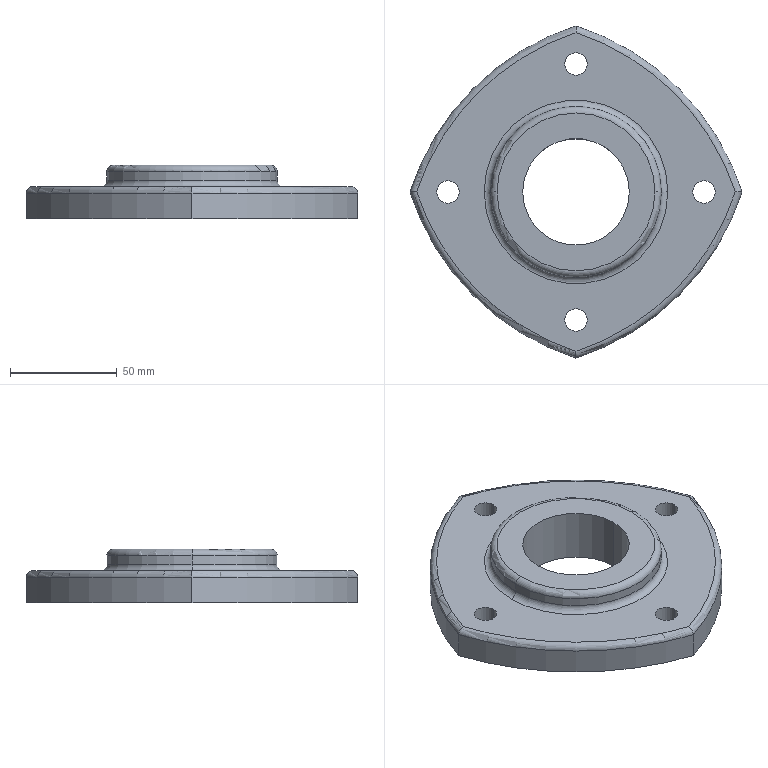Part | SolidWorks | features ICE 2, Extrusion 1, Fillet 1 | 1 solid | 27 faces | box 155.563 x 155.563 x 25 mm | volume 236034 mm3 | cylinder 16 | torus 8 | plane 3 | commonest cylinder face diameters 10.5 x8 240 x4 50 x2 80 x2
STEP:
#1=CARTESIAN_POINT('',(43.,0.,15.));
#2=VERTEX_POINT('',#1);
#3=CARTESIAN_POINT('',(-43.,0.,15.));
#4=VERTEX_POINT('',#3);
#5=CARTESIAN_POINT('',(0.,0.,15.));
#6=DIRECTION('',(0.,0.,-1.));
#7=DIRECTION('',(-1.,0.,0.));
#8=AXIS2_PLACEMENT_3D('',#5,#6,#7);
#9=CIRCLE('',#8,43.);
#10=EDGE_CURVE('',#2,#4,#9,.T.);
#11=ORIENTED_EDGE('',*,*,#10,.F.);
#12=CARTESIAN_POINT('',(40.,0.,18.));
#13=VERTEX_POINT('',#12);
#14=CARTESIAN_POINT('',(43.,0.,18.));
#15=DIRECTION('',(0.,1.,0.));
#16=DIRECTION('',(-1.,0.,0.));
#17=AXIS2_PLACEMENT_3D('',#14,#15,#16);
#18=CIRCLE('',#17,3.);
#19=EDGE_CURVE('',#2,#13,#18,.T.);
#20=ORIENTED_EDGE('',*,*,#19,.T.);
#21=CARTESIAN_POINT('',(-40.,0.,18.));
#22=VERTEX_POINT('',#21);
#23=CARTESIAN_POINT('',(0.,0.,18.));
#24=DIRECTION('',(0.,0.,1.));
#25=DIRECTION('',(-1.,0.,0.));
#26=AXIS2_PLACEMENT_3D('',#23,#24,#25);
#27=CIRCLE('',#26,40.);
#28=EDGE_CURVE('',#22,#13,#27,.T.);
#29=ORIENTED_EDGE('',*,*,#28,.F.);
#30=CARTESIAN_POINT('',(-43.,0.,18.));
#31=DIRECTION('',(0.,-1.,0.));
#32=DIRECTION('',(0.,0.,-1.));
#33=AXIS2_PLACEMENT_3D('',#30,#31,#32);
#34=CIRCLE('',#33,3.);
#35=EDGE_CURVE('',#4,#22,#34,.T.);
#36=ORIENTED_EDGE('',*,*,#35,.F.);
#37=EDGE_LOOP('',(#11,#20,#29,#36));
#38=FACE_OUTER_BOUND('',#37,.T.);
#39=CARTESIAN_POINT('',(0.,0.,18.));
#40=DIRECTION('',(0.,0.,-1.));
#41=DIRECTION('',(-1.,0.,0.));
#42=AXIS2_PLACEMENT_3D('',#39,#40,#41);
#43=TOROIDAL_SURFACE('',#42,43.,3.);
#44=ADVANCED_FACE('',(#38),#43,.F.);
#45=CARTESIAN_POINT('',(-40.,0.,22.));
#46=VERTEX_POINT('',#45);
#47=CARTESIAN_POINT('',(40.,0.,22.));
#48=VERTEX_POINT('',#47);
#49=CARTESIAN_POINT('',(0.,0.,22.));
#50=DIRECTION('',(0.,0.,-1.));
#51=DIRECTION('',(1.,0.,0.));
#52=AXIS2_PLACEMENT_3D('',#49,#50,#51);
#53=CIRCLE('',#52,40.);
#54=EDGE_CURVE('',#46,#48,#53,.T.);
#55=ORIENTED_EDGE('',*,*,#54,.F.);
#56=CARTESIAN_POINT('',(-37.,0.,25.));
#57=VERTEX_POINT('',#56);
#58=CARTESIAN_POINT('',(-37.,0.,22.));
#59=DIRECTION('',(0.,1.,0.));
#60=DIRECTION('',(-1.,0.,0.));
#61=AXIS2_PLACEMENT_3D('',#58,#59,#60);
#62=CIRCLE('',#61,3.);
#63=EDGE_CURVE('',#46,#57,#62,.T.);
#64=ORIENTED_EDGE('',*,*,#63,.T.);
#65=CARTESIAN_POINT('',(37.,0.,25.));
#66=VERTEX_POINT('',#65);
#67=CARTESIAN_POINT('',(0.,0.,25.));
#68=DIRECTION('',(0.,0.,1.));
#69=DIRECTION('',(1.,0.,0.));
#70=AXIS2_PLACEMENT_3D('',#67,#68,#69);
#71=CIRCLE('',#70,37.);
#72=EDGE_CURVE('',#66,#57,#71,.T.);
#73=ORIENTED_EDGE('',*,*,#72,.F.);
#74=CARTESIAN_POINT('',(37.,0.,22.));
#75=DIRECTION('',(0.,-1.,0.));
#76=DIRECTION('',(0.,0.,-1.));
#77=AXIS2_PLACEMENT_3D('',#74,#75,#76);
#78=CIRCLE('',#77,3.);
#79=EDGE_CURVE('',#48,#66,#78,.T.);
#80=ORIENTED_EDGE('',*,*,#79,.F.);
#81=EDGE_LOOP('',(#55,#64,#73,#80));
#82=FACE_OUTER_BOUND('',#81,.T.);
#83=CARTESIAN_POINT('',(0.,0.,22.));
#84=DIRECTION('',(0.,0.,1.));
#85=DIRECTION('',(1.,0.,0.));
#86=AXIS2_PLACEMENT_3D('',#83,#84,#85);
#87=TOROIDAL_SURFACE('',#86,37.,3.);
#88=ADVANCED_FACE('',(#82),#87,.T.);
#89=CARTESIAN_POINT('',(-25.,0.,0.));
#90=VERTEX_POINT('',#89);
#91=CARTESIAN_POINT('',(25.,0.,0.));
#92=VERTEX_POINT('',#91);
#93=CARTESIAN_POINT('',(0.,0.,0.));
#94=DIRECTION('',(0.,0.,1.));
#95=DIRECTION('',(1.,0.,0.));
#96=AXIS2_PLACEMENT_3D('',#93,#94,#95);
#97=CIRCLE('',#96,25.);
#98=EDGE_CURVE('',#90,#92,#97,.T.);
#99=ORIENTED_EDGE('',*,*,#98,.F.);
#100=CARTESIAN_POINT('',(-25.,0.,25.));
#101=VERTEX_POINT('',#100);
#102=CARTESIAN_POINT('',(-25.,0.,0.));
#103=DIRECTION('',(0.,0.,1.));
#104=VECTOR('',#103,1000.);
#105=LINE('',#102,#104);
#106=EDGE_CURVE('',#90,#101,#105,.T.);
#107=ORIENTED_EDGE('',*,*,#106,.T.);
#108=CARTESIAN_POINT('',(25.,0.,25.));
#109=VERTEX_POINT('',#108);
#110=CARTESIAN_POINT('',(0.,0.,25.));
#111=DIRECTION('',(0.,0.,1.));
#112=DIRECTION('',(1.,0.,0.));
#113=AXIS2_PLACEMENT_3D('',#110,#111,#112);
#114=CIRCLE('',#113,25.);
#115=EDGE_CURVE('',#101,#109,#114,.T.);
#116=ORIENTED_EDGE('',*,*,#115,.T.);
#117=CARTESIAN_POINT('',(25.,0.,0.));
#118=DIRECTION('',(0.,0.,1.));
#119=VECTOR('',#118,1000.);
#120=LINE('',#117,#119);
#121=EDGE_CURVE('',#92,#109,#120,.T.);
#122=ORIENTED_EDGE('',*,*,#121,.F.);
#123=EDGE_LOOP('',(#99,#107,#116,#122));
#124=FACE_OUTER_BOUND('',#123,.T.);
#125=CARTESIAN_POINT('',(0.,0.,0.));
#126=DIRECTION('',(0.,0.,1.));
#127=DIRECTION('',(1.,0.,0.));
#128=AXIS2_PLACEMENT_3D('',#125,#126,#127);
#129=CYLINDRICAL_SURFACE('',#128,25.);
#130=ADVANCED_FACE('',(#124),#129,.F.);
#131=ORIENTED_EDGE('',*,*,#54,.T.);
#132=CARTESIAN_POINT('',(40.,0.,25.));
#133=DIRECTION('',(0.,0.,-1.));
#134=VECTOR('',#133,1000.);
#135=LINE('',#132,#134);
#136=EDGE_CURVE('',#48,#13,#135,.T.);
#137=ORIENTED_EDGE('',*,*,#136,.T.);
#138=CARTESIAN_POINT('',(0.,0.,18.));
#139=DIRECTION('',(0.,0.,1.));
#140=DIRECTION('',(-1.,0.,0.));
#141=AXIS2_PLACEMENT_3D('',#138,#139,#140);
#142=CIRCLE('',#141,40.);
#143=EDGE_CURVE('',#13,#22,#142,.T.);
#144=ORIENTED_EDGE('',*,*,#143,.T.);
#145=CARTESIAN_POINT('',(-40.,0.,25.));
#146=DIRECTION('',(0.,0.,-1.));
#147=VECTOR('',#146,1000.);
#148=LINE('',#145,#147);
#149=EDGE_CURVE('',#46,#22,#148,.T.);
#150=ORIENTED_EDGE('',*,*,#149,.F.);
#151=EDGE_LOOP('',(#131,#137,#144,#150));
#152=FACE_OUTER_BOUND('',#151,.T.);
#153=CARTESIAN_POINT('',(0.,0.,25.));
#154=DIRECTION('',(0.,0.,-1.));
#155=DIRECTION('',(-1.,0.,0.));
#156=AXIS2_PLACEMENT_3D('',#153,#154,#155);
#157=CYLINDRICAL_SURFACE('',#156,40.);
#158=ADVANCED_FACE('',(#152),#157,.T.);
#159=CARTESIAN_POINT('',(-65.25,0.,15.));
#160=VERTEX_POINT('',#159);
#161=CARTESIAN_POINT('',(-54.75,0.,15.));
#162=VERTEX_POINT('',#161);
#163=CARTESIAN_POINT('',(-60.,0.,15.));
#164=DIRECTION('',(0.,0.,1.));
#165=DIRECTION('',(1.,0.,0.));
#166=AXIS2_PLACEMENT_3D('',#163,#164,#165);
#167=CIRCLE('',#166,5.25);
#168=EDGE_CURVE('',#160,#162,#167,.T.);
#169=ORIENTED_EDGE('',*,*,#168,.T.);
#170=CARTESIAN_POINT('',(-54.75,0.,0.));
#171=VERTEX_POINT('',#170);
#172=CARTESIAN_POINT('',(-54.75,0.,15.));
#173=DIRECTION('',(0.,0.,-1.));
#174=VECTOR('',#173,1000.);
#175=LINE('',#172,#174);
#176=EDGE_CURVE('',#162,#171,#175,.T.);
#177=ORIENTED_EDGE('',*,*,#176,.T.);
#178=CARTESIAN_POINT('',(-65.25,0.,0.));
#179=VERTEX_POINT('',#178);
#180=CARTESIAN_POINT('',(-60.,0.,0.));
#181=DIRECTION('',(0.,0.,1.));
#182=DIRECTION('',(1.,0.,0.));
#183=AXIS2_PLACEMENT_3D('',#180,#181,#182);
#184=CIRCLE('',#183,5.25);
#185=EDGE_CURVE('',#179,#171,#184,.T.);
#186=ORIENTED_EDGE('',*,*,#185,.F.);
#187=CARTESIAN_POINT('',(-65.25,0.,15.));
#188=DIRECTION('',(0.,0.,-1.));
#189=VECTOR('',#188,1000.);
#190=LINE('',#187,#189);
#191=EDGE_CURVE('',#160,#179,#190,.T.);
#192=ORIENTED_EDGE('',*,*,#191,.F.);
#193=EDGE_LOOP('',(#169,#177,#186,#192));
#194=FACE_OUTER_BOUND('',#193,.T.);
#195=CARTESIAN_POINT('',(-60.,0.,15.));
#196=DIRECTION('',(0.,0.,-1.));
#197=DIRECTION('',(-1.,0.,0.));
#198=AXIS2_PLACEMENT_3D('',#195,#196,#197);
#199=CYLINDRICAL_SURFACE('',#198,5.25);
#200=ADVANCED_FACE('',(#194),#199,.F.);
#201=CARTESIAN_POINT('',(-5.25,-60.,15.));
#202=VERTEX_POINT('',#201);
#203=CARTESIAN_POINT('',(5.25,-60.,15.));
#204=VERTEX_POINT('',#203);
#205=CARTESIAN_POINT('',(0.,-60.,15.));
#206=DIRECTION('',(0.,0.,1.));
#207=DIRECTION('',(1.,0.,0.));
#208=AXIS2_PLACEMENT_3D('',#205,#206,#207);
#209=CIRCLE('',#208,5.25);
#210=EDGE_CURVE('',#202,#204,#209,.T.);
#211=ORIENTED_EDGE('',*,*,#210,.T.);
#212=CARTESIAN_POINT('',(5.25,-60.,0.));
#213=VERTEX_POINT('',#212);
#214=CARTESIAN_POINT('',(5.25,-60.,15.));
#215=DIRECTION('',(0.,0.,-1.));
#216=VECTOR('',#215,1000.);
#217=LINE('',#214,#216);
#218=EDGE_CURVE('',#204,#213,#217,.T.);
#219=ORIENTED_EDGE('',*,*,#218,.T.);
#220=CARTESIAN_POINT('',(-5.25,-60.,0.));
#221=VERTEX_POINT('',#220);
#222=CARTESIAN_POINT('',(0.,-60.,0.));
#223=DIRECTION('',(0.,0.,1.));
#224=DIRECTION('',(1.,0.,0.));
#225=AXIS2_PLACEMENT_3D('',#222,#223,#224);
#226=CIRCLE('',#225,5.25);
#227=EDGE_CURVE('',#221,#213,#226,.T.);
#228=ORIENTED_EDGE('',*,*,#227,.F.);
#229=CARTESIAN_POINT('',(-5.25,-60.,15.));
#230=DIRECTION('',(0.,0.,-1.));
#231=VECTOR('',#230,1000.);
#232=LINE('',#229,#231);
#233=EDGE_CURVE('',#202,#221,#232,.T.);
#234=ORIENTED_EDGE('',*,*,#233,.F.);
#235=EDGE_LOOP('',(#211,#219,#228,#234));
#236=FACE_OUTER_BOUND('',#235,.T.);
#237=CARTESIAN_POINT('',(0.,-60.,15.));
#238=DIRECTION('',(0.,0.,-1.));
#239=DIRECTION('',(-1.,0.,0.));
#240=AXIS2_PLACEMENT_3D('',#237,#238,#239);
#241=CYLINDRICAL_SURFACE('',#240,5.25);
#242=ADVANCED_FACE('',(#236),#241,.F.);
#243=CARTESIAN_POINT('',(54.75,0.,15.));
#244=VERTEX_POINT('',#243);
#245=CARTESIAN_POINT('',(65.25,0.,15.));
#246=VERTEX_POINT('',#245);
#247=CARTESIAN_POINT('',(60.,0.,15.));
#248=DIRECTION('',(0.,0.,1.));
#249=DIRECTION('',(1.,0.,0.));
#250=AXIS2_PLACEMENT_3D('',#247,#248,#249);
#251=CIRCLE('',#250,5.25);
#252=EDGE_CURVE('',#244,#246,#251,.T.);
#253=ORIENTED_EDGE('',*,*,#252,.T.);
#254=CARTESIAN_POINT('',(65.25,0.,0.));
#255=VERTEX_POINT('',#254);
#256=CARTESIAN_POINT('',(65.25,0.,15.));
#257=DIRECTION('',(0.,0.,-1.));
#258=VECTOR('',#257,1000.);
#259=LINE('',#256,#258);
#260=EDGE_CURVE('',#246,#255,#259,.T.);
#261=ORIENTED_EDGE('',*,*,#260,.T.);
#262=CARTESIAN_POINT('',(54.75,0.,0.));
#263=VERTEX_POINT('',#262);
#264=CARTESIAN_POINT('',(60.,0.,0.));
#265=DIRECTION('',(0.,0.,1.));
#266=DIRECTION('',(1.,0.,0.));
#267=AXIS2_PLACEMENT_3D('',#264,#265,#266);
#268=CIRCLE('',#267,5.25);
#269=EDGE_CURVE('',#263,#255,#268,.T.);
#270=ORIENTED_EDGE('',*,*,#269,.F.);
#271=CARTESIAN_POINT('',(54.75,0.,15.));
#272=DIRECTION('',(0.,0.,-1.));
#273=VECTOR('',#272,1000.);
#274=LINE('',#271,#273);
#275=EDGE_CURVE('',#244,#263,#274,.T.);
#276=ORIENTED_EDGE('',*,*,#275,.F.);
#277=EDGE_LOOP('',(#253,#261,#270,#276));
#278=FACE_OUTER_BOUND('',#277,.T.);
#279=CARTESIAN_POINT('',(60.,0.,15.));
#280=DIRECTION('',(0.,0.,-1.));
#281=DIRECTION('',(-1.,0.,0.));
#282=AXIS2_PLACEMENT_3D('',#279,#280,#281);
#283=CYLINDRICAL_SURFACE('',#282,5.25);
#284=ADVANCED_FACE('',(#278),#283,.F.);
#285=CARTESIAN_POINT('',(-5.25,60.,15.));
#286=VERTEX_POINT('',#285);
#287=CARTESIAN_POINT('',(5.25,60.,15.));
#288=VERTEX_POINT('',#287);
#289=CARTESIAN_POINT('',(0.,60.,15.));
#290=DIRECTION('',(0.,0.,1.));
#291=DIRECTION('',(1.,0.,0.));
#292=AXIS2_PLACEMENT_3D('',#289,#290,#291);
#293=CIRCLE('',#292,5.25);
#294=EDGE_CURVE('',#286,#288,#293,.T.);
#295=ORIENTED_EDGE('',*,*,#294,.T.);
#296=CARTESIAN_POINT('',(5.25,60.,0.));
#297=VERTEX_POINT('',#296);
#298=CARTESIAN_POINT('',(5.25,60.,15.));
#299=DIRECTION('',(0.,0.,-1.));
#300=VECTOR('',#299,1000.);
#301=LINE('',#298,#300);
#302=EDGE_CURVE('',#288,#297,#301,.T.);
#303=ORIENTED_EDGE('',*,*,#302,.T.);
#304=CARTESIAN_POINT('',(-5.25,60.,0.));
#305=VERTEX_POINT('',#304);
#306=CARTESIAN_POINT('',(0.,60.,0.));
#307=DIRECTION('',(0.,0.,1.));
#308=DIRECTION('',(1.,0.,0.));
#309=AXIS2_PLACEMENT_3D('',#306,#307,#308);
#310=CIRCLE('',#309,5.25);
#311=EDGE_CURVE('',#305,#297,#310,.T.);
#312=ORIENTED_EDGE('',*,*,#311,.F.);
#313=CARTESIAN_POINT('',(-5.25,60.,15.));
#314=DIRECTION('',(0.,0.,-1.));
#315=VECTOR('',#314,1000.);
#316=LINE('',#313,#315);
#317=EDGE_CURVE('',#286,#305,#316,.T.);
#318=ORIENTED_EDGE('',*,*,#317,.F.);
#319=EDGE_LOOP('',(#295,#303,#312,#318));
#320=FACE_OUTER_BOUND('',#319,.T.);
#321=CARTESIAN_POINT('',(0.,60.,15.));
#322=DIRECTION('',(0.,0.,-1.));
#323=DIRECTION('',(-1.,0.,0.));
#324=AXIS2_PLACEMENT_3D('',#321,#322,#323);
#325=CYLINDRICAL_SURFACE('',#324,5.25);
#326=ADVANCED_FACE('',(#320),#325,.F.);
#327=CARTESIAN_POINT('',(74.628,0.,15.));
#328=VERTEX_POINT('',#327);
#329=CARTESIAN_POINT('',(0.,74.628,15.));
#330=VERTEX_POINT('',#329);
#331=CARTESIAN_POINT('',(-36.525,-36.525,15.));
#332=DIRECTION('',(0.,0.,1.));
#333=DIRECTION('',(-1.,0.,0.));
#334=AXIS2_PLACEMENT_3D('',#331,#332,#333);
#335=CIRCLE('',#334,117.);
#336=EDGE_CURVE('',#328,#330,#335,.T.);
#337=ORIENTED_EDGE('',*,*,#336,.T.);
#338=CARTESIAN_POINT('',(-74.628,0.,15.));
#339=VERTEX_POINT('',#338);
#340=CARTESIAN_POINT('',(36.525,-36.525,15.));
#341=DIRECTION('',(0.,0.,1.));
#342=DIRECTION('',(-1.,0.,0.));
#343=AXIS2_PLACEMENT_3D('',#340,#341,#342);
#344=CIRCLE('',#343,117.);
#345=EDGE_CURVE('',#330,#339,#344,.T.);
#346=ORIENTED_EDGE('',*,*,#345,.T.);
#347=CARTESIAN_POINT('',(0.,-74.628,15.));
#348=VERTEX_POINT('',#347);
#349=CARTESIAN_POINT('',(36.525,36.525,15.));
#350=DIRECTION('',(0.,0.,1.));
#351=DIRECTION('',(-1.,0.,0.));
#352=AXIS2_PLACEMENT_3D('',#349,#350,#351);
#353=CIRCLE('',#352,117.);
#354=EDGE_CURVE('',#339,#348,#353,.T.);
#355=ORIENTED_EDGE('',*,*,#354,.T.);
#356=CARTESIAN_POINT('',(-36.525,36.525,15.));
#357=DIRECTION('',(0.,0.,1.));
#358=DIRECTION('',(-1.,0.,0.));
#359=AXIS2_PLACEMENT_3D('',#356,#357,#358);
#360=CIRCLE('',#359,117.);
#361=EDGE_CURVE('',#348,#328,#360,.T.);
#362=ORIENTED_EDGE('',*,*,#361,.T.);
#363=EDGE_LOOP('',(#337,#346,#355,#362));
#364=FACE_OUTER_BOUND('',#363,.T.);
#365=CARTESIAN_POINT('',(0.,0.,15.));
#366=DIRECTION('',(0.,0.,-1.));
#367=DIRECTION('',(-1.,0.,0.));
#368=AXIS2_PLACEMENT_3D('',#365,#366,#367);
#369=CIRCLE('',#368,43.);
#370=EDGE_CURVE('',#4,#2,#369,.T.);
#371=ORIENTED_EDGE('',*,*,#370,.T.);
#372=ORIENTED_EDGE('',*,*,#10,.T.);
#373=EDGE_LOOP('',(#371,#372));
#374=FACE_BOUND('',#373,.T.);
#375=ORIENTED_EDGE('',*,*,#294,.F.);
#376=CARTESIAN_POINT('',(0.,60.,15.));
#377=DIRECTION('',(0.,0.,1.));
#378=DIRECTION('',(1.,0.,0.));
#379=AXIS2_PLACEMENT_3D('',#376,#377,#378);
#380=CIRCLE('',#379,5.25);
#381=EDGE_CURVE('',#288,#286,#380,.T.);
#382=ORIENTED_EDGE('',*,*,#381,.F.);
#383=EDGE_LOOP('',(#375,#382));
#384=FACE_BOUND('',#383,.T.);
#385=ORIENTED_EDGE('',*,*,#252,.F.);
#386=CARTESIAN_POINT('',(60.,0.,15.));
#387=DIRECTION('',(0.,0.,1.));
#388=DIRECTION('',(1.,0.,0.));
#389=AXIS2_PLACEMENT_3D('',#386,#387,#388);
#390=CIRCLE('',#389,5.25);
#391=EDGE_CURVE('',#246,#244,#390,.T.);
#392=ORIENTED_EDGE('',*,*,#391,.F.);
#393=EDGE_LOOP('',(#385,#392));
#394=FACE_BOUND('',#393,.T.);
#395=ORIENTED_EDGE('',*,*,#210,.F.);
#396=CARTESIAN_POINT('',(0.,-60.,15.));
#397=DIRECTION('',(0.,0.,1.));
#398=DIRECTION('',(1.,0.,0.));
#399=AXIS2_PLACEMENT_3D('',#396,#397,#398);
#400=CIRCLE('',#399,5.25);
#401=EDGE_CURVE('',#204,#202,#400,.T.);
#402=ORIENTED_EDGE('',*,*,#401,.F.);
#403=EDGE_LOOP('',(#395,#402));
#404=FACE_BOUND('',#403,.T.);
#405=ORIENTED_EDGE('',*,*,#168,.F.);
#406=CARTESIAN_POINT('',(-60.,0.,15.));
#407=DIRECTION('',(0.,0.,1.));
#408=DIRECTION('',(1.,0.,0.));
#409=AXIS2_PLACEMENT_3D('',#406,#407,#408);
#410=CIRCLE('',#409,5.25);
#411=EDGE_CURVE('',#162,#160,#410,.T.);
#412=ORIENTED_EDGE('',*,*,#411,.F.);
#413=EDGE_LOOP('',(#405,#412));
#414=FACE_BOUND('',#413,.T.);
#415=CARTESIAN_POINT('',(0.,-36.525,15.));
#416=DIRECTION('',(0.,0.,-1.));
#417=DIRECTION('',(-1.,0.,0.));
#418=AXIS2_PLACEMENT_3D('',#415,#416,#417);
#419=PLANE('',#418);
#420=ADVANCED_FACE('',(#364,#374,#384,#394,#404,#414),#419,.F.);
#421=CARTESIAN_POINT('',(0.,0.,0.));
#422=DIRECTION('',(0.,0.,1.));
#423=DIRECTION('',(1.,0.,0.));
#424=AXIS2_PLACEMENT_3D('',#421,#422,#423);
#425=CIRCLE('',#424,25.);
#426=EDGE_CURVE('',#92,#90,#425,.T.);
#427=ORIENTED_EDGE('',*,*,#426,.T.);
#428=ORIENTED_EDGE('',*,*,#98,.T.);
#429=EDGE_LOOP('',(#427,#428));
#430=FACE_BOUND('',#429,.T.);
#431=ORIENTED_EDGE('',*,*,#227,.T.);
#432=CARTESIAN_POINT('',(0.,-60.,0.));
#433=DIRECTION('',(0.,0.,1.));
#434=DIRECTION('',(1.,0.,0.));
#435=AXIS2_PLACEMENT_3D('',#432,#433,#434);
#436=CIRCLE('',#435,5.25);
#437=EDGE_CURVE('',#213,#221,#436,.T.);
#438=ORIENTED_EDGE('',*,*,#437,.T.);
#439=EDGE_LOOP('',(#431,#438));
#440=FACE_BOUND('',#439,.T.);
#441=ORIENTED_EDGE('',*,*,#311,.T.);
#442=CARTESIAN_POINT('',(0.,60.,0.));
#443=DIRECTION('',(0.,0.,1.));
#444=DIRECTION('',(1.,0.,0.));
#445=AXIS2_PLACEMENT_3D('',#442,#443,#444);
#446=CIRCLE('',#445,5.25);
#447=EDGE_CURVE('',#297,#305,#446,.T.);
#448=ORIENTED_EDGE('',*,*,#447,.T.);
#449=EDGE_LOOP('',(#441,#448));
#450=FACE_BOUND('',#449,.T.);
#451=CARTESIAN_POINT('',(0.,77.782,0.));
#452=VERTEX_POINT('',#451);
#453=CARTESIAN_POINT('',(-77.782,0.,0.));
#454=VERTEX_POINT('',#453);
#455=CARTESIAN_POINT('',(36.525,-36.525,0.));
#456=DIRECTION('',(0.,0.,1.));
#457=DIRECTION('',(-1.,0.,0.));
#458=AXIS2_PLACEMENT_3D('',#455,#456,#457);
#459=CIRCLE('',#458,120.);
#460=EDGE_CURVE('',#452,#454,#459,.T.);
#461=ORIENTED_EDGE('',*,*,#460,.F.);
#462=CARTESIAN_POINT('',(77.782,0.,0.));
#463=VERTEX_POINT('',#462);
#464=CARTESIAN_POINT('',(-36.525,-36.525,0.));
#465=DIRECTION('',(0.,0.,1.));
#466=DIRECTION('',(-1.,0.,0.));
#467=AXIS2_PLACEMENT_3D('',#464,#465,#466);
#468=CIRCLE('',#467,120.);
#469=EDGE_CURVE('',#463,#452,#468,.T.);
#470=ORIENTED_EDGE('',*,*,#469,.F.);
#471=CARTESIAN_POINT('',(0.,-77.782,0.));
#472=VERTEX_POINT('',#471);
#473=CARTESIAN_POINT('',(-36.525,36.525,0.));
#474=DIRECTION('',(0.,0.,1.));
#475=DIRECTION('',(1.,0.,0.));
#476=AXIS2_PLACEMENT_3D('',#473,#474,#475);
#477=CIRCLE('',#476,120.);
#478=EDGE_CURVE('',#472,#463,#477,.T.);
#479=ORIENTED_EDGE('',*,*,#478,.F.);
#480=CARTESIAN_POINT('',(36.525,36.525,0.));
#481=DIRECTION('',(0.,0.,1.));
#482=DIRECTION('',(1.,0.,0.));
#483=AXIS2_PLACEMENT_3D('',#480,#481,#482);
#484=CIRCLE('',#483,120.);
#485=EDGE_CURVE('',#454,#472,#484,.T.);
#486=ORIENTED_EDGE('',*,*,#485,.F.);
#487=EDGE_LOOP('',(#461,#470,#479,#486));
#488=FACE_OUTER_BOUND('',#487,.T.);
#489=ORIENTED_EDGE('',*,*,#269,.T.);
#490=CARTESIAN_POINT('',(60.,0.,0.));
#491=DIRECTION('',(0.,0.,1.));
#492=DIRECTION('',(1.,0.,0.));
#493=AXIS2_PLACEMENT_3D('',#490,#491,#492);
#494=CIRCLE('',#493,5.25);
#495=EDGE_CURVE('',#255,#263,#494,.T.);
#496=ORIENTED_EDGE('',*,*,#495,.T.);
#497=EDGE_LOOP('',(#489,#496));
#498=FACE_BOUND('',#497,.T.);
#499=ORIENTED_EDGE('',*,*,#185,.T.);
#500=CARTESIAN_POINT('',(-60.,0.,0.));
#501=DIRECTION('',(0.,0.,1.));
#502=DIRECTION('',(1.,0.,0.));
#503=AXIS2_PLACEMENT_3D('',#500,#501,#502);
#504=CIRCLE('',#503,5.25);
#505=EDGE_CURVE('',#171,#179,#504,.T.);
#506=ORIENTED_EDGE('',*,*,#505,.T.);
#507=EDGE_LOOP('',(#499,#506));
#508=FACE_BOUND('',#507,.T.);
#509=CARTESIAN_POINT('',(0.,-36.525,0.));
#510=DIRECTION('',(0.,0.,-1.));
#511=DIRECTION('',(-1.,0.,0.));
#512=AXIS2_PLACEMENT_3D('',#509,#510,#511);
#513=PLANE('',#512);
#514=ADVANCED_FACE('',(#430,#440,#450,#488,#498,#508),#513,.T.);
#515=CARTESIAN_POINT('',(-77.782,0.,12.));
#516=VERTEX_POINT('',#515);
#517=CARTESIAN_POINT('',(-77.782,0.,15.));
#518=DIRECTION('',(0.,0.,-1.));
#519=VECTOR('',#518,1000.);
#520=LINE('',#517,#519);
#521=EDGE_CURVE('',#516,#454,#520,.T.);
#522=ORIENTED_EDGE('',*,*,#521,.F.);
#523=CARTESIAN_POINT('',(0.,77.782,12.));
#524=VERTEX_POINT('',#523);
#525=CARTESIAN_POINT('',(36.525,-36.525,12.));
#526=DIRECTION('',(0.,0.,-1.));
#527=DIRECTION('',(-1.,0.,0.));
#528=AXIS2_PLACEMENT_3D('',#525,#526,#527);
#529=CIRCLE('',#528,120.);
#530=EDGE_CURVE('',#516,#524,#529,.T.);
#531=ORIENTED_EDGE('',*,*,#530,.T.);
#532=CARTESIAN_POINT('',(0.,77.782,15.));
#533=DIRECTION('',(0.,0.,-1.));
#534=VECTOR('',#533,1000.);
#535=LINE('',#532,#534);
#536=EDGE_CURVE('',#524,#452,#535,.T.);
#537=ORIENTED_EDGE('',*,*,#536,.T.);
#538=ORIENTED_EDGE('',*,*,#460,.T.);
#539=EDGE_LOOP('',(#522,#531,#537,#538));
#540=FACE_OUTER_BOUND('',#539,.T.);
#541=CARTESIAN_POINT('',(36.525,-36.525,15.));
#542=DIRECTION('',(0.,0.,-1.));
#543=DIRECTION('',(-1.,0.,0.));
#544=AXIS2_PLACEMENT_3D('',#541,#542,#543);
#545=CYLINDRICAL_SURFACE('',#544,120.);
#546=ADVANCED_FACE('',(#540),#545,.T.);
#547=CARTESIAN_POINT('',(0.,-77.782,12.));
#548=VERTEX_POINT('',#547);
#549=CARTESIAN_POINT('',(0.,-77.782,15.));
#550=DIRECTION('',(0.,0.,-1.));
#551=VECTOR('',#550,1000.);
#552=LINE('',#549,#551);
#553=EDGE_CURVE('',#548,#472,#552,.T.);
#554=ORIENTED_EDGE('',*,*,#553,.F.);
#555=CARTESIAN_POINT('',(36.525,36.525,12.));
#556=DIRECTION('',(0.,0.,-1.));
#557=DIRECTION('',(-1.,0.,0.));
#558=AXIS2_PLACEMENT_3D('',#555,#556,#557);
#559=CIRCLE('',#558,120.);
#560=EDGE_CURVE('',#548,#516,#559,.T.);
#561=ORIENTED_EDGE('',*,*,#560,.T.);
#562=ORIENTED_EDGE('',*,*,#521,.T.);
#563=ORIENTED_EDGE('',*,*,#485,.T.);
#564=EDGE_LOOP('',(#554,#561,#562,#563));
#565=FACE_OUTER_BOUND('',#564,.T.);
#566=CARTESIAN_POINT('',(36.525,36.525,15.));
#567=DIRECTION('',(0.,0.,-1.));
#568=DIRECTION('',(-1.,0.,0.));
#569=AXIS2_PLACEMENT_3D('',#566,#567,#568);
#570=CYLINDRICAL_SURFACE('',#569,120.);
#571=ADVANCED_FACE('',(#565),#570,.T.);
#572=CARTESIAN_POINT('',(77.782,0.,12.));
#573=VERTEX_POINT('',#572);
#574=CARTESIAN_POINT('',(77.782,0.,15.));
#575=DIRECTION('',(0.,0.,-1.));
#576=VECTOR('',#575,1000.);
#577=LINE('',#574,#576);
#578=EDGE_CURVE('',#573,#463,#577,.T.);
#579=ORIENTED_EDGE('',*,*,#578,.F.);
#580=CARTESIAN_POINT('',(-36.525,36.525,12.));
#581=DIRECTION('',(0.,0.,-1.));
#582=DIRECTION('',(-1.,0.,0.));
#583=AXIS2_PLACEMENT_3D('',#580,#581,#582);
#584=CIRCLE('',#583,120.);
#585=EDGE_CURVE('',#573,#548,#584,.T.);
#586=ORIENTED_EDGE('',*,*,#585,.T.);
#587=ORIENTED_EDGE('',*,*,#553,.T.);
#588=ORIENTED_EDGE('',*,*,#478,.T.);
#589=EDGE_LOOP('',(#579,#586,#587,#588));
#590=FACE_OUTER_BOUND('',#589,.T.);
#591=CARTESIAN_POINT('',(-36.525,36.525,15.));
#592=DIRECTION('',(0.,0.,-1.));
#593=DIRECTION('',(-1.,0.,0.));
#594=AXIS2_PLACEMENT_3D('',#591,#592,#593);
#595=CYLINDRICAL_SURFACE('',#594,120.);
#596=ADVANCED_FACE('',(#590),#595,.T.);
#597=ORIENTED_EDGE('',*,*,#536,.F.);
#598=CARTESIAN_POINT('',(-36.525,-36.525,12.));
#599=DIRECTION('',(0.,0.,-1.));
#600=DIRECTION('',(-1.,0.,0.));
#601=AXIS2_PLACEMENT_3D('',#598,#599,#600);
#602=CIRCLE('',#601,120.);
#603=EDGE_CURVE('',#524,#573,#602,.T.);
#604=ORIENTED_EDGE('',*,*,#603,.T.);
#605=ORIENTED_EDGE('',*,*,#578,.T.);
#606=ORIENTED_EDGE('',*,*,#469,.T.);
#607=EDGE_LOOP('',(#597,#604,#605,#606));
#608=FACE_OUTER_BOUND('',#607,.T.);
#609=CARTESIAN_POINT('',(-36.525,-36.525,15.));
#610=DIRECTION('',(0.,0.,-1.));
#611=DIRECTION('',(-1.,0.,0.));
#612=AXIS2_PLACEMENT_3D('',#609,#610,#611);
#613=CYLINDRICAL_SURFACE('',#612,120.);
#614=ADVANCED_FACE('',(#608),#613,.T.);
#615=ORIENTED_EDGE('',*,*,#302,.F.);
#616=ORIENTED_EDGE('',*,*,#381,.T.);
#617=ORIENTED_EDGE('',*,*,#317,.T.);
#618=ORIENTED_EDGE('',*,*,#447,.F.);
#619=EDGE_LOOP('',(#615,#616,#617,#618));
#620=FACE_OUTER_BOUND('',#619,.T.);
#621=CARTESIAN_POINT('',(0.,60.,15.));
#622=DIRECTION('',(0.,0.,-1.));
#623=DIRECTION('',(-1.,0.,0.));
#624=AXIS2_PLACEMENT_3D('',#621,#622,#623);
#625=CYLINDRICAL_SURFACE('',#624,5.25);
#626=ADVANCED_FACE('',(#620),#625,.F.);
#627=ORIENTED_EDGE('',*,*,#260,.F.);
#628=ORIENTED_EDGE('',*,*,#391,.T.);
#629=ORIENTED_EDGE('',*,*,#275,.T.);
#630=ORIENTED_EDGE('',*,*,#495,.F.);
#631=EDGE_LOOP('',(#627,#628,#629,#630));
#632=FACE_OUTER_BOUND('',#631,.T.);
#633=CARTESIAN_POINT('',(60.,0.,15.));
#634=DIRECTION('',(0.,0.,-1.));
#635=DIRECTION('',(-1.,0.,0.));
#636=AXIS2_PLACEMENT_3D('',#633,#634,#635);
#637=CYLINDRICAL_SURFACE('',#636,5.25);
#638=ADVANCED_FACE('',(#632),#637,.F.);
#639=ORIENTED_EDGE('',*,*,#218,.F.);
#640=ORIENTED_EDGE('',*,*,#401,.T.);
#641=ORIENTED_EDGE('',*,*,#233,.T.);
#642=ORIENTED_EDGE('',*,*,#437,.F.);
#643=EDGE_LOOP('',(#639,#640,#641,#642));
#644=FACE_OUTER_BOUND('',#643,.T.);
#645=CARTESIAN_POINT('',(0.,-60.,15.));
#646=DIRECTION('',(0.,0.,-1.));
#647=DIRECTION('',(-1.,0.,0.));
#648=AXIS2_PLACEMENT_3D('',#645,#646,#647);
#649=CYLINDRICAL_SURFACE('',#648,5.25);
#650=ADVANCED_FACE('',(#644),#649,.F.);
#651=ORIENTED_EDGE('',*,*,#176,.F.);
#652=ORIENTED_EDGE('',*,*,#411,.T.);
#653=ORIENTED_EDGE('',*,*,#191,.T.);
#654=ORIENTED_EDGE('',*,*,#505,.F.);
#655=EDGE_LOOP('',(#651,#652,#653,#654));
#656=FACE_OUTER_BOUND('',#655,.T.);
#657=CARTESIAN_POINT('',(-60.,0.,15.));
#658=DIRECTION('',(0.,0.,-1.));
#659=DIRECTION('',(-1.,0.,0.));
#660=AXIS2_PLACEMENT_3D('',#657,#658,#659);
#661=CYLINDRICAL_SURFACE('',#660,5.25);
#662=ADVANCED_FACE('',(#656),#661,.F.);
#663=ORIENTED_EDGE('',*,*,#136,.F.);
#664=CARTESIAN_POINT('',(0.,0.,22.));
#665=DIRECTION('',(0.,0.,-1.));
#666=DIRECTION('',(1.,0.,0.));
#667=AXIS2_PLACEMENT_3D('',#664,#665,#666);
#668=CIRCLE('',#667,40.);
#669=EDGE_CURVE('',#48,#46,#668,.T.);
#670=ORIENTED_EDGE('',*,*,#669,.T.);
#671=ORIENTED_EDGE('',*,*,#149,.T.);
#672=ORIENTED_EDGE('',*,*,#28,.T.);
#673=EDGE_LOOP('',(#663,#670,#671,#672));
#674=FACE_OUTER_BOUND('',#673,.T.);
#675=CARTESIAN_POINT('',(0.,0.,25.));
#676=DIRECTION('',(0.,0.,-1.));
#677=DIRECTION('',(-1.,0.,0.));
#678=AXIS2_PLACEMENT_3D('',#675,#676,#677);
#679=CYLINDRICAL_SURFACE('',#678,40.);
#680=ADVANCED_FACE('',(#674),#679,.T.);
#681=ORIENTED_EDGE('',*,*,#72,.T.);
#682=CARTESIAN_POINT('',(0.,0.,25.));
#683=DIRECTION('',(0.,0.,1.));
#684=DIRECTION('',(1.,0.,0.));
#685=AXIS2_PLACEMENT_3D('',#682,#683,#684);
#686=CIRCLE('',#685,37.);
#687=EDGE_CURVE('',#57,#66,#686,.T.);
#688=ORIENTED_EDGE('',*,*,#687,.T.);
#689=EDGE_LOOP('',(#681,#688));
#690=FACE_OUTER_BOUND('',#689,.T.);
#691=CARTESIAN_POINT('',(0.,0.,25.));
#692=DIRECTION('',(0.,0.,1.));
#693=DIRECTION('',(1.,0.,0.));
#694=AXIS2_PLACEMENT_3D('',#691,#692,#693);
#695=CIRCLE('',#694,25.);
#696=EDGE_CURVE('',#109,#101,#695,.T.);
#697=ORIENTED_EDGE('',*,*,#696,.F.);
#698=ORIENTED_EDGE('',*,*,#115,.F.);
#699=EDGE_LOOP('',(#697,#698));
#700=FACE_BOUND('',#699,.T.);
#701=CARTESIAN_POINT('',(0.,0.,25.));
#702=DIRECTION('',(0.,0.,1.));
#703=DIRECTION('',(1.,0.,0.));
#704=AXIS2_PLACEMENT_3D('',#701,#702,#703);
#705=PLANE('',#704);
#706=ADVANCED_FACE('',(#690,#700),#705,.T.);
#707=ORIENTED_EDGE('',*,*,#106,.F.);
#708=ORIENTED_EDGE('',*,*,#426,.F.);
#709=ORIENTED_EDGE('',*,*,#121,.T.);
#710=ORIENTED_EDGE('',*,*,#696,.T.);
#711=EDGE_LOOP('',(#707,#708,#709,#710));
#712=FACE_OUTER_BOUND('',#711,.T.);
#713=CARTESIAN_POINT('',(0.,0.,0.));
#714=DIRECTION('',(0.,0.,1.));
#715=DIRECTION('',(1.,0.,0.));
#716=AXIS2_PLACEMENT_3D('',#713,#714,#715);
#717=CYLINDRICAL_SURFACE('',#716,25.);
#718=ADVANCED_FACE('',(#712),#717,.F.);
#719=CARTESIAN_POINT('',(0.,-77.782,12.));
#720=CARTESIAN_POINT('',(0.,-77.782,12.203));
#721=CARTESIAN_POINT('',(0.,-77.76,12.403));
#722=CARTESIAN_POINT('',(0.,-77.676,12.795));
#723=CARTESIAN_POINT('',(0.,-77.613,12.99));
#724=CARTESIAN_POINT('',(0.,-77.449,13.357));
#725=CARTESIAN_POINT('',(0.,-77.349,13.531));
#726=CARTESIAN_POINT('',(0.,-77.113,13.858));
#727=CARTESIAN_POINT('',(0.,-76.978,14.011));
#728=CARTESIAN_POINT('',(0.,-76.684,14.284));
#729=CARTESIAN_POINT('',(0.,-76.523,14.407));
#730=CARTESIAN_POINT('',(0.,-76.179,14.62));
#731=CARTESIAN_POINT('',(0.,-75.999,14.709));
#732=CARTESIAN_POINT('',(0.,-75.625,14.853));
#733=CARTESIAN_POINT('',(0.,-75.428,14.908));
#734=CARTESIAN_POINT('',(0.,-75.131,14.963));
#735=CARTESIAN_POINT('',(0.,-75.031,14.977));
#736=CARTESIAN_POINT('',(0.,-74.83,14.995));
#737=CARTESIAN_POINT('',(0.,-74.728,15.));
#738=CARTESIAN_POINT('',(0.,-74.628,15.));
#739=B_SPLINE_CURVE_WITH_KNOTS('',3,(#719,#720,#721,#722,#723,#724,#725,#726,#727,#728,#729,#730,#731,#732,#733,#734,#735,#736,#737,#738),.UNSPECIFIED.,.F.,.F.,(4,2,2,2,2,2,2,2,2,4),(0.,0.000601,0.001202,0.001803,0.002404,0.003005,0.003606,0.004207,0.004507,0.004808),.UNSPECIFIED.);
#740=EDGE_CURVE('',#548,#348,#739,.T.);
#741=ORIENTED_EDGE('',*,*,#740,.F.);
#742=ORIENTED_EDGE('',*,*,#585,.F.);
#743=CARTESIAN_POINT('',(74.628,0.,15.));
#744=CARTESIAN_POINT('',(75.031,0.,15.));
#745=CARTESIAN_POINT('',(75.438,0.,14.925));
#746=CARTESIAN_POINT('',(76.,0.,14.709));
#747=CARTESIAN_POINT('',(76.179,0.,14.62));
#748=CARTESIAN_POINT('',(76.523,0.,14.407));
#749=CARTESIAN_POINT('',(76.684,0.,14.284));
#750=CARTESIAN_POINT('',(76.978,0.,14.011));
#751=CARTESIAN_POINT('',(77.113,0.,13.858));
#752=CARTESIAN_POINT('',(77.349,0.,13.531));
#753=CARTESIAN_POINT('',(77.449,0.,13.357));
#754=CARTESIAN_POINT('',(77.613,0.,12.99));
#755=CARTESIAN_POINT('',(77.676,0.,12.795));
#756=CARTESIAN_POINT('',(77.76,0.,12.403));
#757=CARTESIAN_POINT('',(77.782,0.,12.203));
#758=CARTESIAN_POINT('',(77.782,0.,12.));
#759=B_SPLINE_CURVE_WITH_KNOTS('',3,(#743,#744,#745,#746,#747,#748,#749,#750,#751,#752,#753,#754,#755,#756,#757,#758),.UNSPECIFIED.,.F.,.F.,(4,2,2,2,2,2,2,4),(-0.00001422,0.001194,0.001798,0.002403,0.003007,0.003611,0.004215,0.004819),.UNSPECIFIED.);
#760=EDGE_CURVE('',#328,#573,#759,.T.);
#761=ORIENTED_EDGE('',*,*,#760,.F.);
#762=ORIENTED_EDGE('',*,*,#361,.F.);
#763=EDGE_LOOP('',(#741,#742,#761,#762));
#764=FACE_OUTER_BOUND('',#763,.T.);
#765=CARTESIAN_POINT('',(-36.525,36.525,12.));
#766=DIRECTION('',(0.,0.,-1.));
#767=DIRECTION('',(-1.,0.,0.));
#768=AXIS2_PLACEMENT_3D('',#765,#766,#767);
#769=TOROIDAL_SURFACE('',#768,117.,3.);
#770=ADVANCED_FACE('',(#764),#769,.T.);
#771=ORIENTED_EDGE('',*,*,#760,.T.);
#772=ORIENTED_EDGE('',*,*,#603,.F.);
#773=CARTESIAN_POINT('',(0.,74.628,15.));
#774=CARTESIAN_POINT('',(0.,75.031,15.));
#775=CARTESIAN_POINT('',(0.,75.438,14.925));
#776=CARTESIAN_POINT('',(0.,76.,14.709));
#777=CARTESIAN_POINT('',(0.,76.179,14.62));
#778=CARTESIAN_POINT('',(0.,76.523,14.407));
#779=CARTESIAN_POINT('',(0.,76.684,14.284));
#780=CARTESIAN_POINT('',(0.,76.978,14.011));
#781=CARTESIAN_POINT('',(0.,77.113,13.858));
#782=CARTESIAN_POINT('',(0.,77.349,13.531));
#783=CARTESIAN_POINT('',(0.,77.449,13.357));
#784=CARTESIAN_POINT('',(0.,77.613,12.99));
#785=CARTESIAN_POINT('',(0.,77.676,12.795));
#786=CARTESIAN_POINT('',(0.,77.76,12.403));
#787=CARTESIAN_POINT('',(0.,77.782,12.203));
#788=CARTESIAN_POINT('',(0.,77.782,12.));
#789=B_SPLINE_CURVE_WITH_KNOTS('',3,(#773,#774,#775,#776,#777,#778,#779,#780,#781,#782,#783,#784,#785,#786,#787,#788),.UNSPECIFIED.,.F.,.F.,(4,2,2,2,2,2,2,4),(-0.00001422,0.001194,0.001798,0.002403,0.003007,0.003611,0.004215,0.004819),.UNSPECIFIED.);
#790=EDGE_CURVE('',#330,#524,#789,.T.);
#791=ORIENTED_EDGE('',*,*,#790,.F.);
#792=ORIENTED_EDGE('',*,*,#336,.F.);
#793=EDGE_LOOP('',(#771,#772,#791,#792));
#794=FACE_OUTER_BOUND('',#793,.T.);
#795=CARTESIAN_POINT('',(-36.525,-36.525,12.));
#796=DIRECTION('',(0.,0.,-1.));
#797=DIRECTION('',(-1.,0.,0.));
#798=AXIS2_PLACEMENT_3D('',#795,#796,#797);
#799=TOROIDAL_SURFACE('',#798,117.,3.);
#800=ADVANCED_FACE('',(#794),#799,.T.);
#801=ORIENTED_EDGE('',*,*,#740,.T.);
#802=ORIENTED_EDGE('',*,*,#354,.F.);
#803=CARTESIAN_POINT('',(-77.782,0.,12.));
#804=CARTESIAN_POINT('',(-77.782,0.,12.203));
#805=CARTESIAN_POINT('',(-77.76,0.,12.403));
#806=CARTESIAN_POINT('',(-77.676,0.,12.795));
#807=CARTESIAN_POINT('',(-77.613,0.,12.99));
#808=CARTESIAN_POINT('',(-77.449,0.,13.357));
#809=CARTESIAN_POINT('',(-77.349,0.,13.531));
#810=CARTESIAN_POINT('',(-77.113,0.,13.858));
#811=CARTESIAN_POINT('',(-76.978,0.,14.011));
#812=CARTESIAN_POINT('',(-76.684,0.,14.284));
#813=CARTESIAN_POINT('',(-76.523,0.,14.407));
#814=CARTESIAN_POINT('',(-76.179,0.,14.62));
#815=CARTESIAN_POINT('',(-75.999,0.,14.709));
#816=CARTESIAN_POINT('',(-75.625,0.,14.853));
#817=CARTESIAN_POINT('',(-75.428,0.,14.908));
#818=CARTESIAN_POINT('',(-75.131,0.,14.963));
#819=CARTESIAN_POINT('',(-75.031,0.,14.977));
#820=CARTESIAN_POINT('',(-74.83,0.,14.995));
#821=CARTESIAN_POINT('',(-74.728,0.,15.));
#822=CARTESIAN_POINT('',(-74.628,0.,15.));
#823=B_SPLINE_CURVE_WITH_KNOTS('',3,(#803,#804,#805,#806,#807,#808,#809,#810,#811,#812,#813,#814,#815,#816,#817,#818,#819,#820,#821,#822),.UNSPECIFIED.,.F.,.F.,(4,2,2,2,2,2,2,2,2,4),(0.,0.000601,0.001202,0.001803,0.002404,0.003005,0.003606,0.004207,0.004507,0.004808),.UNSPECIFIED.);
#824=EDGE_CURVE('',#516,#339,#823,.T.);
#825=ORIENTED_EDGE('',*,*,#824,.F.);
#826=ORIENTED_EDGE('',*,*,#560,.F.);
#827=EDGE_LOOP('',(#801,#802,#825,#826));
#828=FACE_OUTER_BOUND('',#827,.T.);
#829=CARTESIAN_POINT('',(36.525,36.525,12.));
#830=DIRECTION('',(0.,0.,-1.));
#831=DIRECTION('',(-1.,0.,0.));
#832=AXIS2_PLACEMENT_3D('',#829,#830,#831);
#833=TOROIDAL_SURFACE('',#832,117.,3.);
#834=ADVANCED_FACE('',(#828),#833,.T.);
#835=ORIENTED_EDGE('',*,*,#790,.T.);
#836=ORIENTED_EDGE('',*,*,#530,.F.);
#837=ORIENTED_EDGE('',*,*,#824,.T.);
#838=ORIENTED_EDGE('',*,*,#345,.F.);
#839=EDGE_LOOP('',(#835,#836,#837,#838));
#840=FACE_OUTER_BOUND('',#839,.T.);
#841=CARTESIAN_POINT('',(36.525,-36.525,12.));
#842=DIRECTION('',(0.,0.,-1.));
#843=DIRECTION('',(-1.,0.,0.));
#844=AXIS2_PLACEMENT_3D('',#841,#842,#843);
#845=TOROIDAL_SURFACE('',#844,117.,3.);
#846=ADVANCED_FACE('',(#840),#845,.T.);
#847=ORIENTED_EDGE('',*,*,#63,.F.);
#848=ORIENTED_EDGE('',*,*,#669,.F.);
#849=ORIENTED_EDGE('',*,*,#79,.T.);
#850=ORIENTED_EDGE('',*,*,#687,.F.);
#851=EDGE_LOOP('',(#847,#848,#849,#850));
#852=FACE_OUTER_BOUND('',#851,.T.);
#853=CARTESIAN_POINT('',(0.,0.,22.));
#854=DIRECTION('',(0.,0.,1.));
#855=DIRECTION('',(1.,0.,0.));
#856=AXIS2_PLACEMENT_3D('',#853,#854,#855);
#857=TOROIDAL_SURFACE('',#856,37.,3.);
#858=ADVANCED_FACE('',(#852),#857,.T.);
#859=ORIENTED_EDGE('',*,*,#19,.F.);
#860=ORIENTED_EDGE('',*,*,#370,.F.);
#861=ORIENTED_EDGE('',*,*,#35,.T.);
#862=ORIENTED_EDGE('',*,*,#143,.F.);
#863=EDGE_LOOP('',(#859,#860,#861,#862));
#864=FACE_OUTER_BOUND('',#863,.T.);
#865=CARTESIAN_POINT('',(0.,0.,18.));
#866=DIRECTION('',(0.,0.,-1.));
#867=DIRECTION('',(-1.,0.,0.));
#868=AXIS2_PLACEMENT_3D('',#865,#866,#867);
#869=TOROIDAL_SURFACE('',#868,43.,3.);
#870=ADVANCED_FACE('',(#864),#869,.F.);
#871=CLOSED_SHELL('',(#44,#88,#130,#158,#200,#242,#284,#326,#420,#514,#546,#571,#596,#614,#626,#638,#650,#662,#680,#706,#718,#770,#800,#834,#846,#858,#870));
#872=MANIFOLD_SOLID_BREP('',#871);
#873=CARTESIAN_POINT('',(0.,0.,0.));
#874=DIRECTION('',(0.,0.,1.));
#875=DIRECTION('',(1.,0.,0.));
#876=AXIS2_PLACEMENT_3D('',#873,#874,#875);
#877=(LENGTH_UNIT()NAMED_UNIT(*)SI_UNIT(.MILLI.,.METRE.));
#878=UNCERTAINTY_MEASURE_WITH_UNIT(LENGTH_MEASURE(0.00001),#877,'','');
#879=(NAMED_UNIT(*)PLANE_ANGLE_UNIT()SI_UNIT($,.RADIAN.));
#880=(NAMED_UNIT(*)SI_UNIT($,.STERADIAN.)SOLID_ANGLE_UNIT());
#881=(GEOMETRIC_REPRESENTATION_CONTEXT(3)GLOBAL_UNCERTAINTY_ASSIGNED_CONTEXT((#878))GLOBAL_UNIT_ASSIGNED_CONTEXT((#877,#879,#880))REPRESENTATION_CONTEXT('',''));
#882=ADVANCED_BREP_SHAPE_REPRESENTATION('',(#872,#876),#881);